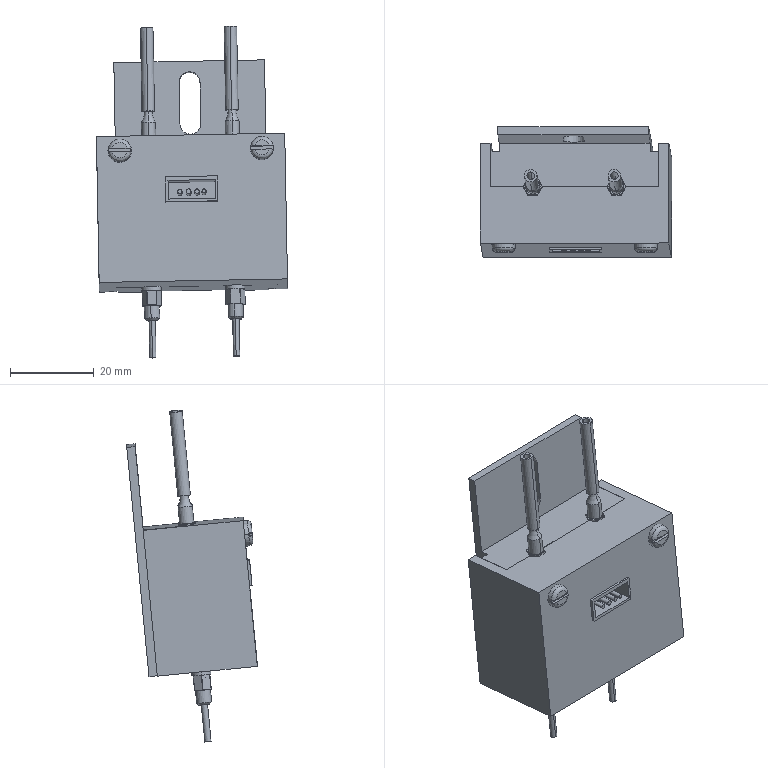Part | SolidWorks | 14 solids | 545 faces | box 45.671 x 31.209 x 79.324 mm | volume 36091 mm3 | plane 249 | cylinder 204 | cone 32 | torus 32 | sphere 28 | commonest cylinder face diameters 0.16 x52 0.2 x32 3 x20 3.6 x16 0.6 x8 1.5 x8